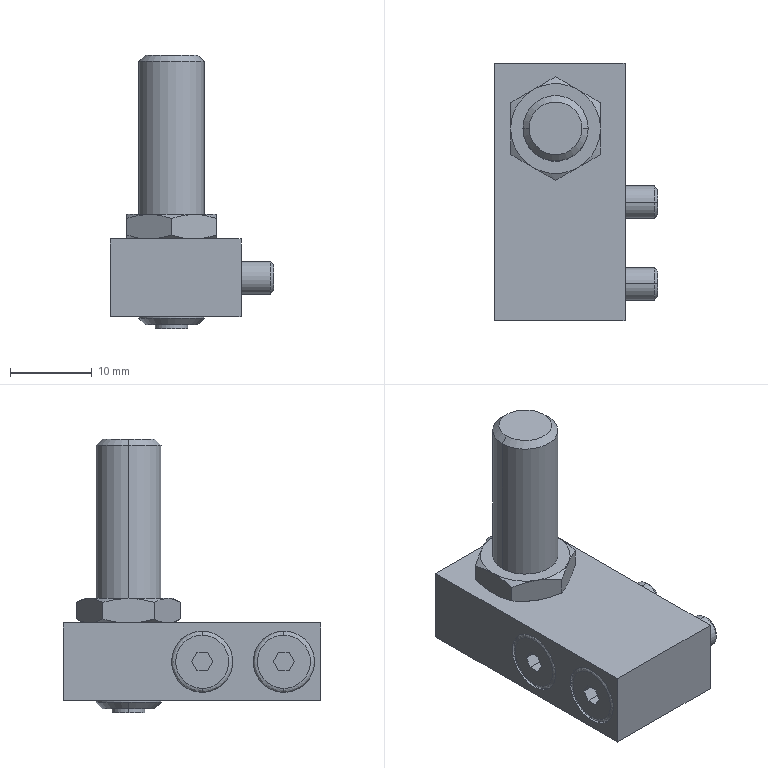Part | STEP file | QA-HI_MDX12_FB | 1 solid | 72 faces | box 20 x 31.5 x 33.5 mm | volume 6201 mm3 | plane 34 | cone 20 | cylinder 14 | spline 4 | commonest cylinder face diameters 4 x6 7.5 x4 8 x4